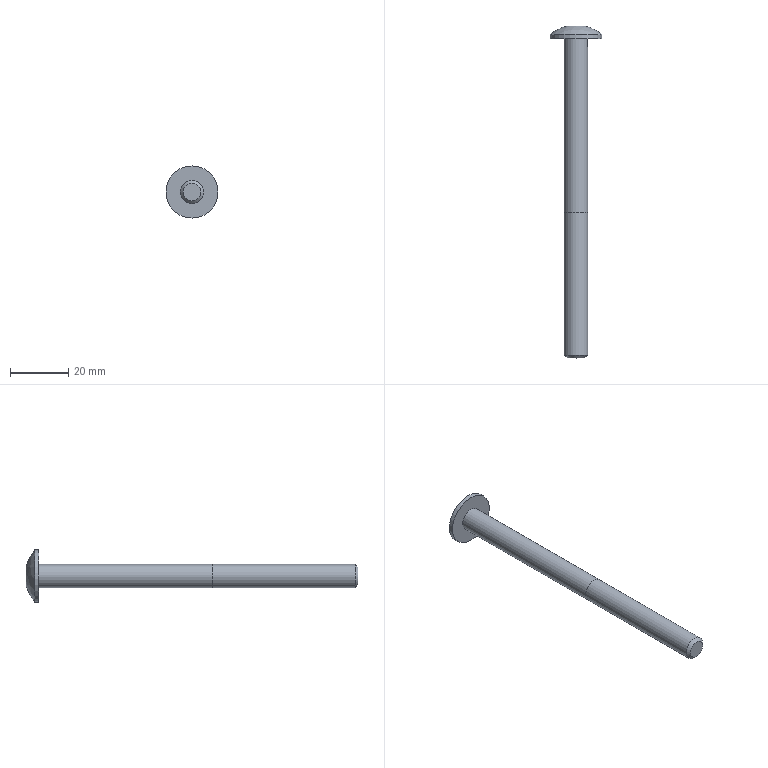Part | STEP file | PN_0020 | 1 solid | 14 faces | box 18 x 114.451 x 18 mm | volume 6223 mm3 | plane 9 | cylinder 3 | sphere 1 | cone 1 | commonest cylinder face diameters 8 x2 18 x1
STEP:
#1=CARTESIAN_POINT('',(0.,0.,0.));
#2=DIRECTION('',(0.,0.,1.));
#3=DIRECTION('',(1.,0.,0.));
#4=AXIS2_PLACEMENT_3D('',#1,#2,#3);
#5=CARTESIAN_POINT('',(0.,0.,4.));
#6=VERTEX_POINT('',#5);
#7=CARTESIAN_POINT('',(0.,0.,0.));
#8=DIRECTION('',(0.,-1.,0.));
#9=DIRECTION('',(0.,0.,1.));
#10=AXIS2_PLACEMENT_3D('',#7,#8,#9);
#11=CIRCLE('',#10,4.);
#12=CARTESIAN_POINT('',(0.,-110.,0.));
#13=DIRECTION('',(0.,1.,0.));
#14=DIRECTION('',(0.,0.,1.));
#15=AXIS2_PLACEMENT_3D('',#12,#13,#14);
#16=CYLINDRICAL_SURFACE('',#15,4.);
#17=CARTESIAN_POINT('',(6.283,110.));
#18=DIRECTION('',(-1.,0.));
#19=VECTOR('',#18,1.);
#20=LINE('',#17,#19);
#21=(GEOMETRIC_REPRESENTATION_CONTEXT(2)PARAMETRIC_REPRESENTATION_CONTEXT()REPRESENTATION_CONTEXT('',''));
#22=DEFINITIONAL_REPRESENTATION('',(#20),#21);
#23=PCURVE('',#16,#22);
#24=CARTESIAN_POINT('',(0.,0.,0.));
#25=DIRECTION('',(0.,1.,0.));
#26=DIRECTION('',(0.,0.,1.));
#27=AXIS2_PLACEMENT_3D('',#24,#25,#26);
#28=PLANE('',#27);
#29=CARTESIAN_POINT('',(4.,0.));
#30=CARTESIAN_POINT('',(4.,-6.928));
#31=CARTESIAN_POINT('',(-2.,-3.464));
#32=CARTESIAN_POINT('',(-8.,0.));
#33=CARTESIAN_POINT('',(-2.,3.464));
#34=CARTESIAN_POINT('',(4.,6.928));
#35=CARTESIAN_POINT('',(4.,0.));
#36=(BOUNDED_CURVE()B_SPLINE_CURVE(2,(#29,#30,#31,#32,#33,#34,#35),.UNSPECIFIED.,.T.,.F.)B_SPLINE_CURVE_WITH_KNOTS((1,2,2,2,2,1),(-2.094,0.,2.094,4.189,6.283,8.378),.UNSPECIFIED.)CURVE()GEOMETRIC_REPRESENTATION_ITEM()RATIONAL_B_SPLINE_CURVE((1.,0.5,1.,0.5,1.,0.5,1.))REPRESENTATION_ITEM(''));
#37=(GEOMETRIC_REPRESENTATION_CONTEXT(2)PARAMETRIC_REPRESENTATION_CONTEXT()REPRESENTATION_CONTEXT('',''));
#38=DEFINITIONAL_REPRESENTATION('',(#36),#37);
#39=PCURVE('',#28,#38);
#40=SURFACE_CURVE('',#11,(#23,#39),.PCURVE_S1.);
#41=EDGE_CURVE('',#6,#6,#40,.T.);
#42=ORIENTED_EDGE('',*,*,#41,.T.);
#43=CARTESIAN_POINT('',(0.,-60.,4.));
#44=VERTEX_POINT('',#43);
#45=CARTESIAN_POINT('',(0.,-60.,4.));
#46=CARTESIAN_POINT('',(0.,0.,4.));
#47=B_SPLINE_CURVE_WITH_KNOTS('',1,(#45,#46),.UNSPECIFIED.,.F.,.F.,(2,2),(50.,110.),.PIECEWISE_BEZIER_KNOTS.);
#48=CARTESIAN_POINT('',(0.,0.));
#49=DIRECTION('',(0.,1.));
#50=VECTOR('',#49,1.);
#51=LINE('',#48,#50);
#52=(GEOMETRIC_REPRESENTATION_CONTEXT(2)PARAMETRIC_REPRESENTATION_CONTEXT()REPRESENTATION_CONTEXT('',''));
#53=DEFINITIONAL_REPRESENTATION('',(#51),#52);
#54=PCURVE('',#16,#53);
#55=CARTESIAN_POINT('',(6.283,0.));
#56=DIRECTION('',(0.,1.));
#57=VECTOR('',#56,1.);
#58=LINE('',#55,#57);
#59=(GEOMETRIC_REPRESENTATION_CONTEXT(2)PARAMETRIC_REPRESENTATION_CONTEXT()REPRESENTATION_CONTEXT('',''));
#60=DEFINITIONAL_REPRESENTATION('',(#58),#59);
#61=PCURVE('',#16,#60);
#62=SEAM_CURVE('',#47,(#54,#61),.PCURVE_S1.);
#63=EDGE_CURVE('',#44,#6,#62,.T.);
#64=ORIENTED_EDGE('',*,*,#63,.F.);
#65=CARTESIAN_POINT('',(0.,-60.,-4.));
#66=VERTEX_POINT('',#65);
#67=CARTESIAN_POINT('',(0.,-60.,0.));
#68=DIRECTION('',(0.,-1.,0.));
#69=DIRECTION('',(0.,0.,-1.));
#70=AXIS2_PLACEMENT_3D('',#67,#68,#69);
#71=CIRCLE('',#70,4.);
#72=CARTESIAN_POINT('',(3.142,50.));
#73=DIRECTION('',(-1.,0.));
#74=VECTOR('',#73,1.);
#75=LINE('',#72,#74);
#76=(GEOMETRIC_REPRESENTATION_CONTEXT(2)PARAMETRIC_REPRESENTATION_CONTEXT()REPRESENTATION_CONTEXT('',''));
#77=DEFINITIONAL_REPRESENTATION('',(#75),#76);
#78=PCURVE('',#16,#77);
#79=CARTESIAN_POINT('',(0.,-110.,0.));
#80=DIRECTION('',(0.,1.,0.));
#81=DIRECTION('',(0.,0.,1.));
#82=AXIS2_PLACEMENT_3D('',#79,#80,#81);
#83=CYLINDRICAL_SURFACE('',#82,4.);
#84=CARTESIAN_POINT('',(9.425,50.));
#85=DIRECTION('',(-1.,0.));
#86=VECTOR('',#85,1.);
#87=LINE('',#84,#86);
#88=(GEOMETRIC_REPRESENTATION_CONTEXT(2)PARAMETRIC_REPRESENTATION_CONTEXT()REPRESENTATION_CONTEXT('',''));
#89=DEFINITIONAL_REPRESENTATION('',(#87),#88);
#90=PCURVE('',#83,#89);
#91=SURFACE_CURVE('',#71,(#78,#90),.PCURVE_S1.);
#92=EDGE_CURVE('',#66,#44,#91,.T.);
#93=ORIENTED_EDGE('',*,*,#92,.F.);
#94=CARTESIAN_POINT('',(0.,-60.,0.));
#95=DIRECTION('',(0.,-1.,0.));
#96=DIRECTION('',(0.,0.,-1.));
#97=AXIS2_PLACEMENT_3D('',#94,#95,#96);
#98=CIRCLE('',#97,4.);
#99=CARTESIAN_POINT('',(9.425,50.));
#100=DIRECTION('',(-1.,0.));
#101=VECTOR('',#100,1.);
#102=LINE('',#99,#101);
#103=(GEOMETRIC_REPRESENTATION_CONTEXT(2)PARAMETRIC_REPRESENTATION_CONTEXT()REPRESENTATION_CONTEXT('',''));
#104=DEFINITIONAL_REPRESENTATION('',(#102),#103);
#105=PCURVE('',#16,#104);
#106=CARTESIAN_POINT('',(9.425,50.));
#107=DIRECTION('',(-1.,0.));
#108=VECTOR('',#107,1.);
#109=LINE('',#106,#108);
#110=(GEOMETRIC_REPRESENTATION_CONTEXT(2)PARAMETRIC_REPRESENTATION_CONTEXT()REPRESENTATION_CONTEXT('',''));
#111=DEFINITIONAL_REPRESENTATION('',(#109),#110);
#112=PCURVE('',#83,#111);
#113=SURFACE_CURVE('',#98,(#105,#112),.PCURVE_S1.);
#114=EDGE_CURVE('',#44,#66,#113,.T.);
#115=ORIENTED_EDGE('',*,*,#114,.F.);
#116=ORIENTED_EDGE('',*,*,#63,.T.);
#117=EDGE_LOOP('',(#42,#64,#93,#115,#116));
#118=FACE_BOUND('',#117,.T.);
#119=ADVANCED_FACE('',(#118),#16,.T.);
#120=CARTESIAN_POINT('',(0.,0.,9.));
#121=VERTEX_POINT('',#120);
#122=CARTESIAN_POINT('',(0.,0.,0.));
#123=DIRECTION('',(0.,1.,0.));
#124=DIRECTION('',(0.,0.,1.));
#125=AXIS2_PLACEMENT_3D('',#122,#123,#124);
#126=CIRCLE('',#125,9.);
#127=CARTESIAN_POINT('',(0.,0.));
#128=DIRECTION('',(1.,0.));
#129=AXIS2_PLACEMENT_2D('',#127,#128);
#130=CIRCLE('',#129,9.);
#131=(GEOMETRIC_REPRESENTATION_CONTEXT(2)PARAMETRIC_REPRESENTATION_CONTEXT()REPRESENTATION_CONTEXT('',''));
#132=DEFINITIONAL_REPRESENTATION('',(#130),#131);
#133=PCURVE('',#28,#132);
#134=CARTESIAN_POINT('',(0.,70.,0.));
#135=DIRECTION('',(0.,1.,0.));
#136=DIRECTION('',(0.,0.,1.));
#137=AXIS2_PLACEMENT_3D('',#134,#135,#136);
#138=CYLINDRICAL_SURFACE('',#137,9.);
#139=CARTESIAN_POINT('',(0.,-70.));
#140=DIRECTION('',(1.,0.));
#141=VECTOR('',#140,1.);
#142=LINE('',#139,#141);
#143=(GEOMETRIC_REPRESENTATION_CONTEXT(2)PARAMETRIC_REPRESENTATION_CONTEXT()REPRESENTATION_CONTEXT('',''));
#144=DEFINITIONAL_REPRESENTATION('',(#142),#143);
#145=PCURVE('',#138,#144);
#146=SURFACE_CURVE('',#126,(#133,#145),.PCURVE_S1.);
#147=EDGE_CURVE('',#121,#121,#146,.T.);
#148=ORIENTED_EDGE('',*,*,#147,.F.);
#149=EDGE_LOOP('',(#148));
#150=FACE_BOUND('',#149,.T.);
#151=ORIENTED_EDGE('',*,*,#41,.F.);
#152=EDGE_LOOP('',(#151));
#153=FACE_BOUND('',#152,.T.);
#154=ADVANCED_FACE('',(#150,#153),#28,.F.);
#155=CARTESIAN_POINT('',(0.,1.5,9.));
#156=VERTEX_POINT('',#155);
#157=CARTESIAN_POINT('',(0.,1.5,0.));
#158=DIRECTION('',(0.,1.,0.));
#159=DIRECTION('',(0.,0.,1.));
#160=AXIS2_PLACEMENT_3D('',#157,#158,#159);
#161=CIRCLE('',#160,9.);
#162=CARTESIAN_POINT('',(0.,-9.224,0.));
#163=DIRECTION('',(0.,0.,-1.));
#164=DIRECTION('',(1.,0.,0.));
#165=AXIS2_PLACEMENT_3D('',#162,#163,#164);
#166=SPHERICAL_SURFACE('',#165,14.);
#167=CARTESIAN_POINT('',(4.712,-0.6982));
#168=CARTESIAN_POINT('',(4.794,-0.6988));
#169=CARTESIAN_POINT('',(4.951,-0.6746));
#170=CARTESIAN_POINT('',(5.148,-0.5787));
#171=CARTESIAN_POINT('',(5.286,-0.4389));
#172=CARTESIAN_POINT('',(5.372,-0.2727));
#173=CARTESIAN_POINT('',(5.412,-0.09234));
#174=CARTESIAN_POINT('',(5.412,0.09234));
#175=CARTESIAN_POINT('',(5.372,0.2727));
#176=CARTESIAN_POINT('',(5.286,0.439));
#177=CARTESIAN_POINT('',(5.148,0.5786));
#178=CARTESIAN_POINT('',(4.952,0.6749));
#179=CARTESIAN_POINT('',(4.712,0.7099));
#180=CARTESIAN_POINT('',(4.473,0.6749));
#181=CARTESIAN_POINT('',(4.277,0.5786));
#182=CARTESIAN_POINT('',(4.138,0.439));
#183=CARTESIAN_POINT('',(4.053,0.2727));
#184=CARTESIAN_POINT('',(4.012,0.09234));
#185=CARTESIAN_POINT('',(4.012,-0.09234));
#186=CARTESIAN_POINT('',(4.053,-0.2727));
#187=CARTESIAN_POINT('',(4.138,-0.4389));
#188=CARTESIAN_POINT('',(4.277,-0.5787));
#189=CARTESIAN_POINT('',(4.474,-0.6746));
#190=CARTESIAN_POINT('',(4.63,-0.6988));
#191=CARTESIAN_POINT('',(4.712,-0.6982));
#192=B_SPLINE_CURVE_WITH_KNOTS('',3,(#167,#168,#169,#170,#171,#172,#173,#174,#175,#176,#177,#178,#179,#180,#181,#182,#183,#184,#185,#186,#187,#188,#189,#190,#191),.UNSPECIFIED.,.T.,.F.,(4,1,1,1,1,1,1,1,1,1,1,1,1,1,1,1,1,1,1,1,1,1,4),(0.,0.2856,0.5712,0.8568,1.142,1.428,1.714,1.999,2.285,2.57,2.856,3.142,3.427,3.713,3.998,4.284,4.57,4.855,5.141,5.426,5.712,5.998,6.283),.QUASI_UNIFORM_KNOTS.);
#193=(GEOMETRIC_REPRESENTATION_CONTEXT(2)PARAMETRIC_REPRESENTATION_CONTEXT()REPRESENTATION_CONTEXT('',''));
#194=DEFINITIONAL_REPRESENTATION('',(#192),#193);
#195=PCURVE('',#166,#194);
#196=CARTESIAN_POINT('',(0.,-68.5));
#197=DIRECTION('',(1.,0.));
#198=VECTOR('',#197,1.);
#199=LINE('',#196,#198);
#200=(GEOMETRIC_REPRESENTATION_CONTEXT(2)PARAMETRIC_REPRESENTATION_CONTEXT()REPRESENTATION_CONTEXT('',''));
#201=DEFINITIONAL_REPRESENTATION('',(#199),#200);
#202=PCURVE('',#138,#201);
#203=SURFACE_CURVE('',#161,(#195,#202),.PCURVE_S1.);
#204=EDGE_CURVE('',#156,#156,#203,.T.);
#205=ORIENTED_EDGE('',*,*,#204,.T.);
#206=EDGE_LOOP('',(#205));
#207=FACE_BOUND('',#206,.T.);
#208=CARTESIAN_POINT('',(0.,4.341,-3.464));
#209=VERTEX_POINT('',#208);
#210=CARTESIAN_POINT('',(-3.,4.341,-1.732));
#211=VERTEX_POINT('',#210);
#212=CARTESIAN_POINT('',(-1.5,-9.224,-2.598));
#213=DIRECTION('',(0.5,0.,0.866));
#214=DIRECTION('',(0.866,0.,-0.5));
#215=AXIS2_PLACEMENT_3D('',#212,#213,#214);
#216=CIRCLE('',#215,13.675);
#217=CARTESIAN_POINT('',(4.712,0.25));
#218=CARTESIAN_POINT('',(4.709,0.2481));
#219=CARTESIAN_POINT('',(4.702,0.2443));
#220=CARTESIAN_POINT('',(4.692,0.2385));
#221=CARTESIAN_POINT('',(4.682,0.2327));
#222=CARTESIAN_POINT('',(4.673,0.2269));
#223=CARTESIAN_POINT('',(4.663,0.2212));
#224=CARTESIAN_POINT('',(4.653,0.2154));
#225=CARTESIAN_POINT('',(4.643,0.2097));
#226=CARTESIAN_POINT('',(4.633,0.2039));
#227=CARTESIAN_POINT('',(4.623,0.1981));
#228=CARTESIAN_POINT('',(4.613,0.1924));
#229=CARTESIAN_POINT('',(4.603,0.1867));
#230=CARTESIAN_POINT('',(4.593,0.1809));
#231=CARTESIAN_POINT('',(4.583,0.1752));
#232=CARTESIAN_POINT('',(4.574,0.1695));
#233=CARTESIAN_POINT('',(4.564,0.1638));
#234=CARTESIAN_POINT('',(4.554,0.1581));
#235=CARTESIAN_POINT('',(4.544,0.1524));
#236=CARTESIAN_POINT('',(4.534,0.1467));
#237=CARTESIAN_POINT('',(4.524,0.141));
#238=CARTESIAN_POINT('',(4.514,0.1353));
#239=CARTESIAN_POINT('',(4.505,0.1297));
#240=CARTESIAN_POINT('',(4.498,0.1259));
#241=CARTESIAN_POINT('',(4.495,0.124));
#242=B_SPLINE_CURVE_WITH_KNOTS('',3,(#217,#218,#219,#220,#221,#222,#223,#224,#225,#226,#227,#228,#229,#230,#231,#232,#233,#234,#235,#236,#237,#238,#239,#240,#241),.UNSPECIFIED.,.F.,.F.,(4,1,1,1,1,1,1,1,1,1,1,1,1,1,1,1,1,1,1,1,1,1,4),(1.444,1.455,1.467,1.478,1.49,1.502,1.513,1.525,1.536,1.548,1.559,1.571,1.582,1.594,1.605,1.617,1.629,1.64,1.652,1.663,1.675,1.686,1.698),.QUASI_UNIFORM_KNOTS.);
#243=(GEOMETRIC_REPRESENTATION_CONTEXT(2)PARAMETRIC_REPRESENTATION_CONTEXT()REPRESENTATION_CONTEXT('',''));
#244=DEFINITIONAL_REPRESENTATION('',(#242),#243);
#245=PCURVE('',#166,#244);
#246=CARTESIAN_POINT('',(-3.,1.,-1.732));
#247=DIRECTION('',(0.5,0.,0.866));
#248=DIRECTION('',(0.866,0.,-0.5));
#249=AXIS2_PLACEMENT_3D('',#246,#247,#248);
#250=PLANE('',#249);
#251=CARTESIAN_POINT('',(1.732,-10.224));
#252=DIRECTION('',(1.,0.));
#253=AXIS2_PLACEMENT_2D('',#251,#252);
#254=CIRCLE('',#253,13.675);
#255=(GEOMETRIC_REPRESENTATION_CONTEXT(2)PARAMETRIC_REPRESENTATION_CONTEXT()REPRESENTATION_CONTEXT('',''));
#256=DEFINITIONAL_REPRESENTATION('',(#254),#255);
#257=PCURVE('',#250,#256);
#258=SURFACE_CURVE('',#216,(#245,#257),.PCURVE_S1.);
#259=EDGE_CURVE('',#209,#211,#258,.T.);
#260=ORIENTED_EDGE('',*,*,#259,.F.);
#261=CARTESIAN_POINT('',(3.,4.341,-1.732));
#262=VERTEX_POINT('',#261);
#263=CARTESIAN_POINT('',(1.5,-9.224,-2.598));
#264=DIRECTION('',(-0.5,0.,0.866));
#265=DIRECTION('',(0.866,0.,0.5));
#266=AXIS2_PLACEMENT_3D('',#263,#264,#265);
#267=CIRCLE('',#266,13.675);
#268=CARTESIAN_POINT('',(4.93,0.124));
#269=CARTESIAN_POINT('',(4.927,0.1259));
#270=CARTESIAN_POINT('',(4.92,0.1297));
#271=CARTESIAN_POINT('',(4.91,0.1353));
#272=CARTESIAN_POINT('',(4.901,0.141));
#273=CARTESIAN_POINT('',(4.891,0.1467));
#274=CARTESIAN_POINT('',(4.881,0.1524));
#275=CARTESIAN_POINT('',(4.871,0.1581));
#276=CARTESIAN_POINT('',(4.861,0.1638));
#277=CARTESIAN_POINT('',(4.851,0.1695));
#278=CARTESIAN_POINT('',(4.841,0.1752));
#279=CARTESIAN_POINT('',(4.832,0.1809));
#280=CARTESIAN_POINT('',(4.822,0.1867));
#281=CARTESIAN_POINT('',(4.812,0.1924));
#282=CARTESIAN_POINT('',(4.802,0.1981));
#283=CARTESIAN_POINT('',(4.792,0.2039));
#284=CARTESIAN_POINT('',(4.782,0.2097));
#285=CARTESIAN_POINT('',(4.772,0.2154));
#286=CARTESIAN_POINT('',(4.762,0.2212));
#287=CARTESIAN_POINT('',(4.752,0.2269));
#288=CARTESIAN_POINT('',(4.742,0.2327));
#289=CARTESIAN_POINT('',(4.732,0.2385));
#290=CARTESIAN_POINT('',(4.722,0.2443));
#291=CARTESIAN_POINT('',(4.716,0.2481));
#292=CARTESIAN_POINT('',(4.712,0.25));
#293=B_SPLINE_CURVE_WITH_KNOTS('',3,(#268,#269,#270,#271,#272,#273,#274,#275,#276,#277,#278,#279,#280,#281,#282,#283,#284,#285,#286,#287,#288,#289,#290,#291,#292),.UNSPECIFIED.,.F.,.F.,(4,1,1,1,1,1,1,1,1,1,1,1,1,1,1,1,1,1,1,1,1,1,4),(1.444,1.455,1.467,1.478,1.49,1.502,1.513,1.525,1.536,1.548,1.559,1.571,1.582,1.594,1.605,1.617,1.629,1.64,1.652,1.663,1.675,1.686,1.698),.QUASI_UNIFORM_KNOTS.);
#294=(GEOMETRIC_REPRESENTATION_CONTEXT(2)PARAMETRIC_REPRESENTATION_CONTEXT()REPRESENTATION_CONTEXT('',''));
#295=DEFINITIONAL_REPRESENTATION('',(#293),#294);
#296=PCURVE('',#166,#295);
#297=CARTESIAN_POINT('',(0.,1.,-3.464));
#298=DIRECTION('',(-0.5,0.,0.866));
#299=DIRECTION('',(0.866,0.,0.5));
#300=AXIS2_PLACEMENT_3D('',#297,#298,#299);
#301=PLANE('',#300);
#302=CARTESIAN_POINT('',(1.732,-10.224));
#303=DIRECTION('',(1.,0.));
#304=AXIS2_PLACEMENT_2D('',#302,#303);
#305=CIRCLE('',#304,13.675);
#306=(GEOMETRIC_REPRESENTATION_CONTEXT(2)PARAMETRIC_REPRESENTATION_CONTEXT()REPRESENTATION_CONTEXT('',''));
#307=DEFINITIONAL_REPRESENTATION('',(#305),#306);
#308=PCURVE('',#301,#307);
#309=SURFACE_CURVE('',#267,(#296,#308),.PCURVE_S1.);
#310=EDGE_CURVE('',#262,#209,#309,.T.);
#311=ORIENTED_EDGE('',*,*,#310,.F.);
#312=CARTESIAN_POINT('',(3.,4.341,1.732));
#313=VERTEX_POINT('',#312);
#314=CARTESIAN_POINT('',(3.,-9.224,0.));
#315=DIRECTION('',(-1.,0.,0.));
#316=DIRECTION('',(0.,0.,1.));
#317=AXIS2_PLACEMENT_3D('',#314,#315,#316);
#318=CIRCLE('',#317,13.675);
#319=CARTESIAN_POINT('',(4.93,-0.124));
#320=CARTESIAN_POINT('',(4.93,-0.1203));
#321=CARTESIAN_POINT('',(4.93,-0.1128));
#322=CARTESIAN_POINT('',(4.929,-0.1015));
#323=CARTESIAN_POINT('',(4.929,-0.09021));
#324=CARTESIAN_POINT('',(4.929,-0.07894));
#325=CARTESIAN_POINT('',(4.929,-0.06766));
#326=CARTESIAN_POINT('',(4.929,-0.05639));
#327=CARTESIAN_POINT('',(4.929,-0.04511));
#328=CARTESIAN_POINT('',(4.928,-0.03383));
#329=CARTESIAN_POINT('',(4.928,-0.02255));
#330=CARTESIAN_POINT('',(4.928,-0.01128));
#331=CARTESIAN_POINT('',(4.928,0.));
#332=CARTESIAN_POINT('',(4.928,0.01128));
#333=CARTESIAN_POINT('',(4.928,0.02255));
#334=CARTESIAN_POINT('',(4.928,0.03383));
#335=CARTESIAN_POINT('',(4.929,0.04511));
#336=CARTESIAN_POINT('',(4.929,0.05639));
#337=CARTESIAN_POINT('',(4.929,0.06766));
#338=CARTESIAN_POINT('',(4.929,0.07894));
#339=CARTESIAN_POINT('',(4.929,0.09021));
#340=CARTESIAN_POINT('',(4.929,0.1015));
#341=CARTESIAN_POINT('',(4.93,0.1128));
#342=CARTESIAN_POINT('',(4.93,0.1203));
#343=CARTESIAN_POINT('',(4.93,0.124));
#344=B_SPLINE_CURVE_WITH_KNOTS('',3,(#319,#320,#321,#322,#323,#324,#325,#326,#327,#328,#329,#330,#331,#332,#333,#334,#335,#336,#337,#338,#339,#340,#341,#342,#343),.UNSPECIFIED.,.F.,.F.,(4,1,1,1,1,1,1,1,1,1,1,1,1,1,1,1,1,1,1,1,1,1,4),(1.444,1.455,1.467,1.478,1.49,1.502,1.513,1.525,1.536,1.548,1.559,1.571,1.582,1.594,1.605,1.617,1.629,1.64,1.652,1.663,1.675,1.686,1.698),.QUASI_UNIFORM_KNOTS.);
#345=(GEOMETRIC_REPRESENTATION_CONTEXT(2)PARAMETRIC_REPRESENTATION_CONTEXT()REPRESENTATION_CONTEXT('',''));
#346=DEFINITIONAL_REPRESENTATION('',(#344),#345);
#347=PCURVE('',#166,#346);
#348=CARTESIAN_POINT('',(3.,1.,-1.732));
#349=DIRECTION('',(-1.,0.,0.));
#350=DIRECTION('',(0.,0.,1.));
#351=AXIS2_PLACEMENT_3D('',#348,#349,#350);
#352=PLANE('',#351);
#353=CARTESIAN_POINT('',(1.732,-10.224));
#354=DIRECTION('',(1.,0.));
#355=AXIS2_PLACEMENT_2D('',#353,#354);
#356=CIRCLE('',#355,13.675);
#357=(GEOMETRIC_REPRESENTATION_CONTEXT(2)PARAMETRIC_REPRESENTATION_CONTEXT()REPRESENTATION_CONTEXT('',''));
#358=DEFINITIONAL_REPRESENTATION('',(#356),#357);
#359=PCURVE('',#352,#358);
#360=SURFACE_CURVE('',#318,(#347,#359),.PCURVE_S1.);
#361=EDGE_CURVE('',#313,#262,#360,.T.);
#362=ORIENTED_EDGE('',*,*,#361,.F.);
#363=CARTESIAN_POINT('',(0.,4.341,3.464));
#364=VERTEX_POINT('',#363);
#365=CARTESIAN_POINT('',(1.5,-9.224,2.598));
#366=DIRECTION('',(-0.5,0.,-0.866));
#367=DIRECTION('',(-0.866,0.,0.5));
#368=AXIS2_PLACEMENT_3D('',#365,#366,#367);
#369=CIRCLE('',#368,13.675);
#370=CARTESIAN_POINT('',(4.712,-0.25));
#371=CARTESIAN_POINT('',(4.716,-0.2481));
#372=CARTESIAN_POINT('',(4.722,-0.2443));
#373=CARTESIAN_POINT('',(4.732,-0.2385));
#374=CARTESIAN_POINT('',(4.742,-0.2327));
#375=CARTESIAN_POINT('',(4.752,-0.2269));
#376=CARTESIAN_POINT('',(4.762,-0.2212));
#377=CARTESIAN_POINT('',(4.772,-0.2154));
#378=CARTESIAN_POINT('',(4.782,-0.2097));
#379=CARTESIAN_POINT('',(4.792,-0.2039));
#380=CARTESIAN_POINT('',(4.802,-0.1981));
#381=CARTESIAN_POINT('',(4.812,-0.1924));
#382=CARTESIAN_POINT('',(4.822,-0.1867));
#383=CARTESIAN_POINT('',(4.832,-0.1809));
#384=CARTESIAN_POINT('',(4.841,-0.1752));
#385=CARTESIAN_POINT('',(4.851,-0.1695));
#386=CARTESIAN_POINT('',(4.861,-0.1638));
#387=CARTESIAN_POINT('',(4.871,-0.1581));
#388=CARTESIAN_POINT('',(4.881,-0.1524));
#389=CARTESIAN_POINT('',(4.891,-0.1467));
#390=CARTESIAN_POINT('',(4.901,-0.141));
#391=CARTESIAN_POINT('',(4.91,-0.1353));
#392=CARTESIAN_POINT('',(4.92,-0.1297));
#393=CARTESIAN_POINT('',(4.927,-0.1259));
#394=CARTESIAN_POINT('',(4.93,-0.124));
#395=B_SPLINE_CURVE_WITH_KNOTS('',3,(#370,#371,#372,#373,#374,#375,#376,#377,#378,#379,#380,#381,#382,#383,#384,#385,#386,#387,#388,#389,#390,#391,#392,#393,#394),.UNSPECIFIED.,.F.,.F.,(4,1,1,1,1,1,1,1,1,1,1,1,1,1,1,1,1,1,1,1,1,1,4),(1.444,1.455,1.467,1.478,1.49,1.502,1.513,1.525,1.536,1.548,1.559,1.571,1.582,1.594,1.605,1.617,1.629,1.64,1.652,1.663,1.675,1.686,1.698),.QUASI_UNIFORM_KNOTS.);
#396=(GEOMETRIC_REPRESENTATION_CONTEXT(2)PARAMETRIC_REPRESENTATION_CONTEXT()REPRESENTATION_CONTEXT('',''));
#397=DEFINITIONAL_REPRESENTATION('',(#395),#396);
#398=PCURVE('',#166,#397);
#399=CARTESIAN_POINT('',(3.,1.,1.732));
#400=DIRECTION('',(-0.5,0.,-0.866));
#401=DIRECTION('',(-0.866,0.,0.5));
#402=AXIS2_PLACEMENT_3D('',#399,#400,#401);
#403=PLANE('',#402);
#404=CARTESIAN_POINT('',(1.732,-10.224));
#405=DIRECTION('',(1.,0.));
#406=AXIS2_PLACEMENT_2D('',#404,#405);
#407=CIRCLE('',#406,13.675);
#408=(GEOMETRIC_REPRESENTATION_CONTEXT(2)PARAMETRIC_REPRESENTATION_CONTEXT()REPRESENTATION_CONTEXT('',''));
#409=DEFINITIONAL_REPRESENTATION('',(#407),#408);
#410=PCURVE('',#403,#409);
#411=SURFACE_CURVE('',#369,(#398,#410),.PCURVE_S1.);
#412=EDGE_CURVE('',#364,#313,#411,.T.);
#413=ORIENTED_EDGE('',*,*,#412,.F.);
#414=CARTESIAN_POINT('',(-3.,4.341,1.732));
#415=VERTEX_POINT('',#414);
#416=CARTESIAN_POINT('',(-1.5,-9.224,2.598));
#417=DIRECTION('',(0.5,0.,-0.866));
#418=DIRECTION('',(-0.866,0.,-0.5));
#419=AXIS2_PLACEMENT_3D('',#416,#417,#418);
#420=CIRCLE('',#419,13.675);
#421=CARTESIAN_POINT('',(4.495,-0.124));
#422=CARTESIAN_POINT('',(4.498,-0.1259));
#423=CARTESIAN_POINT('',(4.505,-0.1297));
#424=CARTESIAN_POINT('',(4.514,-0.1353));
#425=CARTESIAN_POINT('',(4.524,-0.141));
#426=CARTESIAN_POINT('',(4.534,-0.1467));
#427=CARTESIAN_POINT('',(4.544,-0.1524));
#428=CARTESIAN_POINT('',(4.554,-0.1581));
#429=CARTESIAN_POINT('',(4.564,-0.1638));
#430=CARTESIAN_POINT('',(4.574,-0.1695));
#431=CARTESIAN_POINT('',(4.583,-0.1752));
#432=CARTESIAN_POINT('',(4.593,-0.1809));
#433=CARTESIAN_POINT('',(4.603,-0.1867));
#434=CARTESIAN_POINT('',(4.613,-0.1924));
#435=CARTESIAN_POINT('',(4.623,-0.1981));
#436=CARTESIAN_POINT('',(4.633,-0.2039));
#437=CARTESIAN_POINT('',(4.643,-0.2097));
#438=CARTESIAN_POINT('',(4.653,-0.2154));
#439=CARTESIAN_POINT('',(4.663,-0.2212));
#440=CARTESIAN_POINT('',(4.673,-0.2269));
#441=CARTESIAN_POINT('',(4.682,-0.2327));
#442=CARTESIAN_POINT('',(4.692,-0.2385));
#443=CARTESIAN_POINT('',(4.702,-0.2443));
#444=CARTESIAN_POINT('',(4.709,-0.2481));
#445=CARTESIAN_POINT('',(4.712,-0.25));
#446=B_SPLINE_CURVE_WITH_KNOTS('',3,(#421,#422,#423,#424,#425,#426,#427,#428,#429,#430,#431,#432,#433,#434,#435,#436,#437,#438,#439,#440,#441,#442,#443,#444,#445),.UNSPECIFIED.,.F.,.F.,(4,1,1,1,1,1,1,1,1,1,1,1,1,1,1,1,1,1,1,1,1,1,4),(1.444,1.455,1.467,1.478,1.49,1.502,1.513,1.525,1.536,1.548,1.559,1.571,1.582,1.594,1.605,1.617,1.629,1.64,1.652,1.663,1.675,1.686,1.698),.QUASI_UNIFORM_KNOTS.);
#447=(GEOMETRIC_REPRESENTATION_CONTEXT(2)PARAMETRIC_REPRESENTATION_CONTEXT()REPRESENTATION_CONTEXT('',''));
#448=DEFINITIONAL_REPRESENTATION('',(#446),#447);
#449=PCURVE('',#166,#448);
#450=CARTESIAN_POINT('',(0.,1.,3.464));
#451=DIRECTION('',(0.5,0.,-0.866));
#452=DIRECTION('',(-0.866,0.,-0.5));
#453=AXIS2_PLACEMENT_3D('',#450,#451,#452);
#454=PLANE('',#453);
#455=CARTESIAN_POINT('',(1.732,-10.224));
#456=DIRECTION('',(1.,0.));
#457=AXIS2_PLACEMENT_2D('',#455,#456);
#458=CIRCLE('',#457,13.675);
#459=(GEOMETRIC_REPRESENTATION_CONTEXT(2)PARAMETRIC_REPRESENTATION_CONTEXT()REPRESENTATION_CONTEXT('',''));
#460=DEFINITIONAL_REPRESENTATION('',(#458),#459);
#461=PCURVE('',#454,#460);
#462=SURFACE_CURVE('',#420,(#449,#461),.PCURVE_S1.);
#463=EDGE_CURVE('',#415,#364,#462,.T.);
#464=ORIENTED_EDGE('',*,*,#463,.F.);
#465=CARTESIAN_POINT('',(-3.,-9.224,0.));
#466=DIRECTION('',(1.,0.,0.));
#467=DIRECTION('',(0.,0.,-1.));
#468=AXIS2_PLACEMENT_3D('',#465,#466,#467);
#469=CIRCLE('',#468,13.675);
#470=CARTESIAN_POINT('',(4.495,0.124));
#471=CARTESIAN_POINT('',(4.495,0.1203));
#472=CARTESIAN_POINT('',(4.495,0.1128));
#473=CARTESIAN_POINT('',(4.495,0.1015));
#474=CARTESIAN_POINT('',(4.496,0.09021));
#475=CARTESIAN_POINT('',(4.496,0.07894));
#476=CARTESIAN_POINT('',(4.496,0.06766));
#477=CARTESIAN_POINT('',(4.496,0.05639));
#478=CARTESIAN_POINT('',(4.496,0.04511));
#479=CARTESIAN_POINT('',(4.496,0.03383));
#480=CARTESIAN_POINT('',(4.496,0.02255));
#481=CARTESIAN_POINT('',(4.496,0.01128));
#482=CARTESIAN_POINT('',(4.496,0.));
#483=CARTESIAN_POINT('',(4.496,-0.01128));
#484=CARTESIAN_POINT('',(4.496,-0.02255));
#485=CARTESIAN_POINT('',(4.496,-0.03383));
#486=CARTESIAN_POINT('',(4.496,-0.04511));
#487=CARTESIAN_POINT('',(4.496,-0.05639));
#488=CARTESIAN_POINT('',(4.496,-0.06766));
#489=CARTESIAN_POINT('',(4.496,-0.07894));
#490=CARTESIAN_POINT('',(4.496,-0.09021));
#491=CARTESIAN_POINT('',(4.495,-0.1015));
#492=CARTESIAN_POINT('',(4.495,-0.1128));
#493=CARTESIAN_POINT('',(4.495,-0.1203));
#494=CARTESIAN_POINT('',(4.495,-0.124));
#495=B_SPLINE_CURVE_WITH_KNOTS('',3,(#470,#471,#472,#473,#474,#475,#476,#477,#478,#479,#480,#481,#482,#483,#484,#485,#486,#487,#488,#489,#490,#491,#492,#493,#494),.UNSPECIFIED.,.F.,.F.,(4,1,1,1,1,1,1,1,1,1,1,1,1,1,1,1,1,1,1,1,1,1,4),(1.444,1.455,1.467,1.478,1.49,1.502,1.513,1.525,1.536,1.548,1.559,1.571,1.582,1.594,1.605,1.617,1.629,1.64,1.652,1.663,1.675,1.686,1.698),.QUASI_UNIFORM_KNOTS.);
#496=(GEOMETRIC_REPRESENTATION_CONTEXT(2)PARAMETRIC_REPRESENTATION_CONTEXT()REPRESENTATION_CONTEXT('',''));
#497=DEFINITIONAL_REPRESENTATION('',(#495),#496);
#498=PCURVE('',#166,#497);
#499=CARTESIAN_POINT('',(-3.,1.,1.732));
#500=DIRECTION('',(1.,0.,0.));
#501=DIRECTION('',(0.,0.,-1.));
#502=AXIS2_PLACEMENT_3D('',#499,#500,#501);
#503=PLANE('',#502);
#504=CARTESIAN_POINT('',(1.732,-10.224));
#505=DIRECTION('',(1.,0.));
#506=AXIS2_PLACEMENT_2D('',#504,#505);
#507=CIRCLE('',#506,13.675);
#508=(GEOMETRIC_REPRESENTATION_CONTEXT(2)PARAMETRIC_REPRESENTATION_CONTEXT()REPRESENTATION_CONTEXT('',''));
#509=DEFINITIONAL_REPRESENTATION('',(#507),#508);
#510=PCURVE('',#503,#509);
#511=SURFACE_CURVE('',#469,(#498,#510),.PCURVE_S1.);
#512=EDGE_CURVE('',#211,#415,#511,.T.);
#513=ORIENTED_EDGE('',*,*,#512,.F.);
#514=EDGE_LOOP('',(#260,#311,#362,#413,#464,#513));
#515=FACE_BOUND('',#514,.T.);
#516=ADVANCED_FACE('',(#207,#515),#166,.T.);
#517=ORIENTED_EDGE('',*,*,#204,.F.);
#518=CARTESIAN_POINT('',(0.,0.,9.));
#519=CARTESIAN_POINT('',(0.,1.5,9.));
#520=B_SPLINE_CURVE_WITH_KNOTS('',1,(#518,#519),.UNSPECIFIED.,.F.,.F.,(2,2),(-70.,-68.5),.PIECEWISE_BEZIER_KNOTS.);
#521=CARTESIAN_POINT('',(0.,0.));
#522=DIRECTION('',(0.,1.));
#523=VECTOR('',#522,1.);
#524=LINE('',#521,#523);
#525=(GEOMETRIC_REPRESENTATION_CONTEXT(2)PARAMETRIC_REPRESENTATION_CONTEXT()REPRESENTATION_CONTEXT('',''));
#526=DEFINITIONAL_REPRESENTATION('',(#524),#525);
#527=PCURVE('',#138,#526);
#528=CARTESIAN_POINT('',(6.283,0.));
#529=DIRECTION('',(0.,1.));
#530=VECTOR('',#529,1.);
#531=LINE('',#528,#530);
#532=(GEOMETRIC_REPRESENTATION_CONTEXT(2)PARAMETRIC_REPRESENTATION_CONTEXT()REPRESENTATION_CONTEXT('',''));
#533=DEFINITIONAL_REPRESENTATION('',(#531),#532);
#534=PCURVE('',#138,#533);
#535=SEAM_CURVE('',#520,(#527,#534),.PCURVE_S1.);
#536=EDGE_CURVE('',#121,#156,#535,.T.);
#537=ORIENTED_EDGE('',*,*,#536,.F.);
#538=ORIENTED_EDGE('',*,*,#147,.T.);
#539=ORIENTED_EDGE('',*,*,#536,.T.);
#540=EDGE_LOOP('',(#517,#537,#538,#539));
#541=FACE_BOUND('',#540,.T.);
#542=ADVANCED_FACE('',(#541),#138,.T.);
#543=ORIENTED_EDGE('',*,*,#259,.T.);
#544=CARTESIAN_POINT('',(-3.,1.,-1.732));
#545=VERTEX_POINT('',#544);
#546=CARTESIAN_POINT('',(-3.,1.,-1.732));
#547=DIRECTION('',(0.,1.,0.));
#548=VECTOR('',#547,1.);
#549=LINE('',#546,#548);
#550=CARTESIAN_POINT('',(0.,0.));
#551=DIRECTION('',(0.,1.));
#552=VECTOR('',#551,1.);
#553=LINE('',#550,#552);
#554=(GEOMETRIC_REPRESENTATION_CONTEXT(2)PARAMETRIC_REPRESENTATION_CONTEXT()REPRESENTATION_CONTEXT('',''));
#555=DEFINITIONAL_REPRESENTATION('',(#553),#554);
#556=PCURVE('',#250,#555);
#557=CARTESIAN_POINT('',(3.464,0.));
#558=DIRECTION('',(0.,1.));
#559=VECTOR('',#558,1.);
#560=LINE('',#557,#559);
#561=(GEOMETRIC_REPRESENTATION_CONTEXT(2)PARAMETRIC_REPRESENTATION_CONTEXT()REPRESENTATION_CONTEXT('',''));
#562=DEFINITIONAL_REPRESENTATION('',(#560),#561);
#563=PCURVE('',#503,#562);
#564=SURFACE_CURVE('',#549,(#556,#563),.PCURVE_S1.);
#565=EDGE_CURVE('',#545,#211,#564,.T.);
#566=ORIENTED_EDGE('',*,*,#565,.F.);
#567=CARTESIAN_POINT('',(0.,1.,-3.464));
#568=VERTEX_POINT('',#567);
#569=CARTESIAN_POINT('',(-3.,1.,-1.732));
#570=DIRECTION('',(0.866,0.,-0.5));
#571=VECTOR('',#570,1.);
#572=LINE('',#569,#571);
#573=CARTESIAN_POINT('',(0.,0.));
#574=DIRECTION('',(1.,0.));
#575=VECTOR('',#574,1.);
#576=LINE('',#573,#575);
#577=(GEOMETRIC_REPRESENTATION_CONTEXT(2)PARAMETRIC_REPRESENTATION_CONTEXT()REPRESENTATION_CONTEXT('',''));
#578=DEFINITIONAL_REPRESENTATION('',(#576),#577);
#579=PCURVE('',#250,#578);
#580=CARTESIAN_POINT('',(-3.,1.,-1.732));
#581=DIRECTION('',(0.,1.,0.));
#582=DIRECTION('',(0.,0.,1.));
#583=AXIS2_PLACEMENT_3D('',#580,#581,#582);
#584=PLANE('',#583);
#585=CARTESIAN_POINT('',(0.,0.));
#586=DIRECTION('',(-0.5,0.866));
#587=VECTOR('',#586,1.);
#588=LINE('',#585,#587);
#589=(GEOMETRIC_REPRESENTATION_CONTEXT(2)PARAMETRIC_REPRESENTATION_CONTEXT()REPRESENTATION_CONTEXT('',''));
#590=DEFINITIONAL_REPRESENTATION('',(#588),#589);
#591=PCURVE('',#584,#590);
#592=SURFACE_CURVE('',#572,(#579,#591),.PCURVE_S1.);
#593=EDGE_CURVE('',#545,#568,#592,.T.);
#594=ORIENTED_EDGE('',*,*,#593,.T.);
#595=CARTESIAN_POINT('',(0.,1.,-3.464));
#596=DIRECTION('',(0.,1.,0.));
#597=VECTOR('',#596,1.);
#598=LINE('',#595,#597);
#599=CARTESIAN_POINT('',(3.464,0.));
#600=DIRECTION('',(0.,1.));
#601=VECTOR('',#600,1.);
#602=LINE('',#599,#601);
#603=(GEOMETRIC_REPRESENTATION_CONTEXT(2)PARAMETRIC_REPRESENTATION_CONTEXT()REPRESENTATION_CONTEXT('',''));
#604=DEFINITIONAL_REPRESENTATION('',(#602),#603);
#605=PCURVE('',#250,#604);
#606=CARTESIAN_POINT('',(0.,0.));
#607=DIRECTION('',(0.,1.));
#608=VECTOR('',#607,1.);
#609=LINE('',#606,#608);
#610=(GEOMETRIC_REPRESENTATION_CONTEXT(2)PARAMETRIC_REPRESENTATION_CONTEXT()REPRESENTATION_CONTEXT('',''));
#611=DEFINITIONAL_REPRESENTATION('',(#609),#610);
#612=PCURVE('',#301,#611);
#613=SURFACE_CURVE('',#598,(#605,#612),.PCURVE_S1.);
#614=EDGE_CURVE('',#568,#209,#613,.T.);
#615=ORIENTED_EDGE('',*,*,#614,.T.);
#616=EDGE_LOOP('',(#543,#566,#594,#615));
#617=FACE_BOUND('',#616,.T.);
#618=ADVANCED_FACE('',(#617),#250,.T.);
#619=ORIENTED_EDGE('',*,*,#310,.T.);
#620=ORIENTED_EDGE('',*,*,#614,.F.);
#621=CARTESIAN_POINT('',(3.,1.,-1.732));
#622=VERTEX_POINT('',#621);
#623=CARTESIAN_POINT('',(0.,1.,-3.464));
#624=DIRECTION('',(0.866,0.,0.5));
#625=VECTOR('',#624,1.);
#626=LINE('',#623,#625);
#627=CARTESIAN_POINT('',(0.,0.));
#628=DIRECTION('',(1.,0.));
#629=VECTOR('',#628,1.);
#630=LINE('',#627,#629);
#631=(GEOMETRIC_REPRESENTATION_CONTEXT(2)PARAMETRIC_REPRESENTATION_CONTEXT()REPRESENTATION_CONTEXT('',''));
#632=DEFINITIONAL_REPRESENTATION('',(#630),#631);
#633=PCURVE('',#301,#632);
#634=CARTESIAN_POINT('',(-1.732,3.));
#635=DIRECTION('',(0.5,0.866));
#636=VECTOR('',#635,1.);
#637=LINE('',#634,#636);
#638=(GEOMETRIC_REPRESENTATION_CONTEXT(2)PARAMETRIC_REPRESENTATION_CONTEXT()REPRESENTATION_CONTEXT('',''));
#639=DEFINITIONAL_REPRESENTATION('',(#637),#638);
#640=PCURVE('',#584,#639);
#641=SURFACE_CURVE('',#626,(#633,#640),.PCURVE_S1.);
#642=EDGE_CURVE('',#568,#622,#641,.T.);
#643=ORIENTED_EDGE('',*,*,#642,.T.);
#644=CARTESIAN_POINT('',(3.,1.,-1.732));
#645=DIRECTION('',(0.,1.,0.));
#646=VECTOR('',#645,1.);
#647=LINE('',#644,#646);
#648=CARTESIAN_POINT('',(3.464,0.));
#649=DIRECTION('',(0.,1.));
#650=VECTOR('',#649,1.);
#651=LINE('',#648,#650);
#652=(GEOMETRIC_REPRESENTATION_CONTEXT(2)PARAMETRIC_REPRESENTATION_CONTEXT()REPRESENTATION_CONTEXT('',''));
#653=DEFINITIONAL_REPRESENTATION('',(#651),#652);
#654=PCURVE('',#301,#653);
#655=CARTESIAN_POINT('',(0.,0.));
#656=DIRECTION('',(0.,1.));
#657=VECTOR('',#656,1.);
#658=LINE('',#655,#657);
#659=(GEOMETRIC_REPRESENTATION_CONTEXT(2)PARAMETRIC_REPRESENTATION_CONTEXT()REPRESENTATION_CONTEXT('',''));
#660=DEFINITIONAL_REPRESENTATION('',(#658),#659);
#661=PCURVE('',#352,#660);
#662=SURFACE_CURVE('',#647,(#654,#661),.PCURVE_S1.);
#663=EDGE_CURVE('',#622,#262,#662,.T.);
#664=ORIENTED_EDGE('',*,*,#663,.T.);
#665=EDGE_LOOP('',(#619,#620,#643,#664));
#666=FACE_BOUND('',#665,.T.);
#667=ADVANCED_FACE('',(#666),#301,.T.);
#668=ORIENTED_EDGE('',*,*,#361,.T.);
#669=ORIENTED_EDGE('',*,*,#663,.F.);
#670=CARTESIAN_POINT('',(3.,1.,1.732));
#671=VERTEX_POINT('',#670);
#672=CARTESIAN_POINT('',(3.,1.,-1.732));
#673=DIRECTION('',(0.,0.,1.));
#674=VECTOR('',#673,1.);
#675=LINE('',#672,#674);
#676=CARTESIAN_POINT('',(0.,0.));
#677=DIRECTION('',(1.,0.));
#678=VECTOR('',#677,1.);
#679=LINE('',#676,#678);
#680=(GEOMETRIC_REPRESENTATION_CONTEXT(2)PARAMETRIC_REPRESENTATION_CONTEXT()REPRESENTATION_CONTEXT('',''));
#681=DEFINITIONAL_REPRESENTATION('',(#679),#680);
#682=PCURVE('',#352,#681);
#683=CARTESIAN_POINT('',(0.,6.));
#684=DIRECTION('',(1.,0.));
#685=VECTOR('',#684,1.);
#686=LINE('',#683,#685);
#687=(GEOMETRIC_REPRESENTATION_CONTEXT(2)PARAMETRIC_REPRESENTATION_CONTEXT()REPRESENTATION_CONTEXT('',''));
#688=DEFINITIONAL_REPRESENTATION('',(#686),#687);
#689=PCURVE('',#584,#688);
#690=SURFACE_CURVE('',#675,(#682,#689),.PCURVE_S1.);
#691=EDGE_CURVE('',#622,#671,#690,.T.);
#692=ORIENTED_EDGE('',*,*,#691,.T.);
#693=CARTESIAN_POINT('',(3.,1.,1.732));
#694=DIRECTION('',(0.,1.,0.));
#695=VECTOR('',#694,1.);
#696=LINE('',#693,#695);
#697=CARTESIAN_POINT('',(3.464,0.));
#698=DIRECTION('',(0.,1.));
#699=VECTOR('',#698,1.);
#700=LINE('',#697,#699);
#701=(GEOMETRIC_REPRESENTATION_CONTEXT(2)PARAMETRIC_REPRESENTATION_CONTEXT()REPRESENTATION_CONTEXT('',''));
#702=DEFINITIONAL_REPRESENTATION('',(#700),#701);
#703=PCURVE('',#352,#702);
#704=CARTESIAN_POINT('',(0.,0.));
#705=DIRECTION('',(0.,1.));
#706=VECTOR('',#705,1.);
#707=LINE('',#704,#706);
#708=(GEOMETRIC_REPRESENTATION_CONTEXT(2)PARAMETRIC_REPRESENTATION_CONTEXT()REPRESENTATION_CONTEXT('',''));
#709=DEFINITIONAL_REPRESENTATION('',(#707),#708);
#710=PCURVE('',#403,#709);
#711=SURFACE_CURVE('',#696,(#703,#710),.PCURVE_S1.);
#712=EDGE_CURVE('',#671,#313,#711,.T.);
#713=ORIENTED_EDGE('',*,*,#712,.T.);
#714=EDGE_LOOP('',(#668,#669,#692,#713));
#715=FACE_BOUND('',#714,.T.);
#716=ADVANCED_FACE('',(#715),#352,.T.);
#717=ORIENTED_EDGE('',*,*,#412,.T.);
#718=ORIENTED_EDGE('',*,*,#712,.F.);
#719=CARTESIAN_POINT('',(0.,1.,3.464));
#720=VERTEX_POINT('',#719);
#721=CARTESIAN_POINT('',(3.,1.,1.732));
#722=DIRECTION('',(-0.866,0.,0.5));
#723=VECTOR('',#722,1.);
#724=LINE('',#721,#723);
#725=CARTESIAN_POINT('',(0.,0.));
#726=DIRECTION('',(1.,0.));
#727=VECTOR('',#726,1.);
#728=LINE('',#725,#727);
#729=(GEOMETRIC_REPRESENTATION_CONTEXT(2)PARAMETRIC_REPRESENTATION_CONTEXT()REPRESENTATION_CONTEXT('',''));
#730=DEFINITIONAL_REPRESENTATION('',(#728),#729);
#731=PCURVE('',#403,#730);
#732=CARTESIAN_POINT('',(3.464,6.));
#733=DIRECTION('',(0.5,-0.866));
#734=VECTOR('',#733,1.);
#735=LINE('',#732,#734);
#736=(GEOMETRIC_REPRESENTATION_CONTEXT(2)PARAMETRIC_REPRESENTATION_CONTEXT()REPRESENTATION_CONTEXT('',''));
#737=DEFINITIONAL_REPRESENTATION('',(#735),#736);
#738=PCURVE('',#584,#737);
#739=SURFACE_CURVE('',#724,(#731,#738),.PCURVE_S1.);
#740=EDGE_CURVE('',#671,#720,#739,.T.);
#741=ORIENTED_EDGE('',*,*,#740,.T.);
#742=CARTESIAN_POINT('',(0.,1.,3.464));
#743=DIRECTION('',(0.,1.,0.));
#744=VECTOR('',#743,1.);
#745=LINE('',#742,#744);
#746=CARTESIAN_POINT('',(3.464,0.));
#747=DIRECTION('',(0.,1.));
#748=VECTOR('',#747,1.);
#749=LINE('',#746,#748);
#750=(GEOMETRIC_REPRESENTATION_CONTEXT(2)PARAMETRIC_REPRESENTATION_CONTEXT()REPRESENTATION_CONTEXT('',''));
#751=DEFINITIONAL_REPRESENTATION('',(#749),#750);
#752=PCURVE('',#403,#751);
#753=CARTESIAN_POINT('',(0.,0.));
#754=DIRECTION('',(0.,1.));
#755=VECTOR('',#754,1.);
#756=LINE('',#753,#755);
#757=(GEOMETRIC_REPRESENTATION_CONTEXT(2)PARAMETRIC_REPRESENTATION_CONTEXT()REPRESENTATION_CONTEXT('',''));
#758=DEFINITIONAL_REPRESENTATION('',(#756),#757);
#759=PCURVE('',#454,#758);
#760=SURFACE_CURVE('',#745,(#752,#759),.PCURVE_S1.);
#761=EDGE_CURVE('',#720,#364,#760,.T.);
#762=ORIENTED_EDGE('',*,*,#761,.T.);
#763=EDGE_LOOP('',(#717,#718,#741,#762));
#764=FACE_BOUND('',#763,.T.);
#765=ADVANCED_FACE('',(#764),#403,.T.);
#766=ORIENTED_EDGE('',*,*,#463,.T.);
#767=ORIENTED_EDGE('',*,*,#761,.F.);
#768=CARTESIAN_POINT('',(-3.,1.,1.732));
#769=VERTEX_POINT('',#768);
#770=CARTESIAN_POINT('',(0.,1.,3.464));
#771=DIRECTION('',(-0.866,0.,-0.5));
#772=VECTOR('',#771,1.);
#773=LINE('',#770,#772);
#774=CARTESIAN_POINT('',(0.,0.));
#775=DIRECTION('',(1.,0.));
#776=VECTOR('',#775,1.);
#777=LINE('',#774,#776);
#778=(GEOMETRIC_REPRESENTATION_CONTEXT(2)PARAMETRIC_REPRESENTATION_CONTEXT()REPRESENTATION_CONTEXT('',''));
#779=DEFINITIONAL_REPRESENTATION('',(#777),#778);
#780=PCURVE('',#454,#779);
#781=CARTESIAN_POINT('',(5.196,3.));
#782=DIRECTION('',(-0.5,-0.866));
#783=VECTOR('',#782,1.);
#784=LINE('',#781,#783);
#785=(GEOMETRIC_REPRESENTATION_CONTEXT(2)PARAMETRIC_REPRESENTATION_CONTEXT()REPRESENTATION_CONTEXT('',''));
#786=DEFINITIONAL_REPRESENTATION('',(#784),#785);
#787=PCURVE('',#584,#786);
#788=SURFACE_CURVE('',#773,(#780,#787),.PCURVE_S1.);
#789=EDGE_CURVE('',#720,#769,#788,.T.);
#790=ORIENTED_EDGE('',*,*,#789,.T.);
#791=CARTESIAN_POINT('',(-3.,1.,1.732));
#792=DIRECTION('',(0.,1.,0.));
#793=VECTOR('',#792,1.);
#794=LINE('',#791,#793);
#795=CARTESIAN_POINT('',(3.464,0.));
#796=DIRECTION('',(0.,1.));
#797=VECTOR('',#796,1.);
#798=LINE('',#795,#797);
#799=(GEOMETRIC_REPRESENTATION_CONTEXT(2)PARAMETRIC_REPRESENTATION_CONTEXT()REPRESENTATION_CONTEXT('',''));
#800=DEFINITIONAL_REPRESENTATION('',(#798),#799);
#801=PCURVE('',#454,#800);
#802=CARTESIAN_POINT('',(0.,0.));
#803=DIRECTION('',(0.,1.));
#804=VECTOR('',#803,1.);
#805=LINE('',#802,#804);
#806=(GEOMETRIC_REPRESENTATION_CONTEXT(2)PARAMETRIC_REPRESENTATION_CONTEXT()REPRESENTATION_CONTEXT('',''));
#807=DEFINITIONAL_REPRESENTATION('',(#805),#806);
#808=PCURVE('',#503,#807);
#809=SURFACE_CURVE('',#794,(#801,#808),.PCURVE_S1.);
#810=EDGE_CURVE('',#769,#415,#809,.T.);
#811=ORIENTED_EDGE('',*,*,#810,.T.);
#812=EDGE_LOOP('',(#766,#767,#790,#811));
#813=FACE_BOUND('',#812,.T.);
#814=ADVANCED_FACE('',(#813),#454,.T.);
#815=ORIENTED_EDGE('',*,*,#512,.T.);
#816=ORIENTED_EDGE('',*,*,#810,.F.);
#817=CARTESIAN_POINT('',(-3.,1.,1.732));
#818=DIRECTION('',(0.,0.,-1.));
#819=VECTOR('',#818,1.);
#820=LINE('',#817,#819);
#821=CARTESIAN_POINT('',(0.,0.));
#822=DIRECTION('',(1.,0.));
#823=VECTOR('',#822,1.);
#824=LINE('',#821,#823);
#825=(GEOMETRIC_REPRESENTATION_CONTEXT(2)PARAMETRIC_REPRESENTATION_CONTEXT()REPRESENTATION_CONTEXT('',''));
#826=DEFINITIONAL_REPRESENTATION('',(#824),#825);
#827=PCURVE('',#503,#826);
#828=CARTESIAN_POINT('',(3.464,0.));
#829=DIRECTION('',(-1.,0.));
#830=VECTOR('',#829,1.);
#831=LINE('',#828,#830);
#832=(GEOMETRIC_REPRESENTATION_CONTEXT(2)PARAMETRIC_REPRESENTATION_CONTEXT()REPRESENTATION_CONTEXT('',''));
#833=DEFINITIONAL_REPRESENTATION('',(#831),#832);
#834=PCURVE('',#584,#833);
#835=SURFACE_CURVE('',#820,(#827,#834),.PCURVE_S1.);
#836=EDGE_CURVE('',#769,#545,#835,.T.);
#837=ORIENTED_EDGE('',*,*,#836,.T.);
#838=ORIENTED_EDGE('',*,*,#565,.T.);
#839=EDGE_LOOP('',(#815,#816,#837,#838));
#840=FACE_BOUND('',#839,.T.);
#841=ADVANCED_FACE('',(#840),#503,.T.);
#842=ORIENTED_EDGE('',*,*,#593,.F.);
#843=ORIENTED_EDGE('',*,*,#836,.F.);
#844=ORIENTED_EDGE('',*,*,#789,.F.);
#845=ORIENTED_EDGE('',*,*,#740,.F.);
#846=ORIENTED_EDGE('',*,*,#691,.F.);
#847=ORIENTED_EDGE('',*,*,#642,.F.);
#848=EDGE_LOOP('',(#842,#843,#844,#845,#846,#847));
#849=FACE_BOUND('',#848,.T.);
#850=ADVANCED_FACE('',(#849),#584,.T.);
#851=ORIENTED_EDGE('',*,*,#92,.T.);
#852=ORIENTED_EDGE('',*,*,#114,.T.);
#853=CARTESIAN_POINT('',(0.,-109.,-4.));
#854=VERTEX_POINT('',#853);
#855=CARTESIAN_POINT('',(0.,-109.,-4.));
#856=CARTESIAN_POINT('',(0.,-60.,-4.));
#857=B_SPLINE_CURVE_WITH_KNOTS('',1,(#855,#856),.UNSPECIFIED.,.F.,.F.,(2,2),(1.,50.),.PIECEWISE_BEZIER_KNOTS.);
#858=CARTESIAN_POINT('',(3.142,0.));
#859=DIRECTION('',(0.,1.));
#860=VECTOR('',#859,1.);
#861=LINE('',#858,#860);
#862=(GEOMETRIC_REPRESENTATION_CONTEXT(2)PARAMETRIC_REPRESENTATION_CONTEXT()REPRESENTATION_CONTEXT('',''));
#863=DEFINITIONAL_REPRESENTATION('',(#861),#862);
#864=PCURVE('',#83,#863);
#865=CARTESIAN_POINT('',(9.425,0.));
#866=DIRECTION('',(0.,1.));
#867=VECTOR('',#866,1.);
#868=LINE('',#865,#867);
#869=(GEOMETRIC_REPRESENTATION_CONTEXT(2)PARAMETRIC_REPRESENTATION_CONTEXT()REPRESENTATION_CONTEXT('',''));
#870=DEFINITIONAL_REPRESENTATION('',(#868),#869);
#871=PCURVE('',#83,#870);
#872=SEAM_CURVE('',#857,(#864,#871),.PCURVE_S1.);
#873=EDGE_CURVE('',#854,#66,#872,.T.);
#874=ORIENTED_EDGE('',*,*,#873,.F.);
#875=CARTESIAN_POINT('',(0.,-109.,0.));
#876=DIRECTION('',(0.,1.,0.));
#877=DIRECTION('',(0.,0.,-1.));
#878=AXIS2_PLACEMENT_3D('',#875,#876,#877);
#879=CIRCLE('',#878,4.);
#880=CARTESIAN_POINT('',(3.142,1.));
#881=DIRECTION('',(1.,0.));
#882=VECTOR('',#881,1.);
#883=LINE('',#880,#882);
#884=(GEOMETRIC_REPRESENTATION_CONTEXT(2)PARAMETRIC_REPRESENTATION_CONTEXT()REPRESENTATION_CONTEXT('',''));
#885=DEFINITIONAL_REPRESENTATION('',(#883),#884);
#886=PCURVE('',#83,#885);
#887=CARTESIAN_POINT('',(0.,-110.,0.));
#888=DIRECTION('',(0.,1.,0.));
#889=DIRECTION('',(0.,0.,1.));
#890=AXIS2_PLACEMENT_3D('',#887,#888,#889);
#891=CONICAL_SURFACE('',#890,3.,0.7854);
#892=CARTESIAN_POINT('',(3.142,1.));
#893=DIRECTION('',(1.,0.));
#894=VECTOR('',#893,1.);
#895=LINE('',#892,#894);
#896=(GEOMETRIC_REPRESENTATION_CONTEXT(2)PARAMETRIC_REPRESENTATION_CONTEXT()REPRESENTATION_CONTEXT('',''));
#897=DEFINITIONAL_REPRESENTATION('',(#895),#896);
#898=PCURVE('',#891,#897);
#899=SURFACE_CURVE('',#879,(#886,#898),.PCURVE_S1.);
#900=EDGE_CURVE('',#854,#854,#899,.T.);
#901=ORIENTED_EDGE('',*,*,#900,.T.);
#902=ORIENTED_EDGE('',*,*,#873,.T.);
#903=EDGE_LOOP('',(#851,#852,#874,#901,#902));
#904=FACE_BOUND('',#903,.T.);
#905=ADVANCED_FACE('',(#904),#83,.T.);
#906=CARTESIAN_POINT('',(0.,-110.,-3.));
#907=VERTEX_POINT('',#906);
#908=CARTESIAN_POINT('',(0.,-110.,0.));
#909=DIRECTION('',(0.,-1.,0.));
#910=DIRECTION('',(0.,0.,-1.));
#911=AXIS2_PLACEMENT_3D('',#908,#909,#910);
#912=CIRCLE('',#911,3.);
#913=CARTESIAN_POINT('',(0.,-110.,0.));
#914=DIRECTION('',(0.,-1.,0.));
#915=DIRECTION('',(0.,0.,-1.));
#916=AXIS2_PLACEMENT_3D('',#913,#914,#915);
#917=PLANE('',#916);
#918=CARTESIAN_POINT('',(0.,0.));
#919=DIRECTION('',(1.,0.));
#920=AXIS2_PLACEMENT_2D('',#918,#919);
#921=CIRCLE('',#920,3.);
#922=(GEOMETRIC_REPRESENTATION_CONTEXT(2)PARAMETRIC_REPRESENTATION_CONTEXT()REPRESENTATION_CONTEXT('',''));
#923=DEFINITIONAL_REPRESENTATION('',(#921),#922);
#924=PCURVE('',#917,#923);
#925=CARTESIAN_POINT('',(9.425,0.));
#926=DIRECTION('',(-1.,0.));
#927=VECTOR('',#926,1.);
#928=LINE('',#925,#927);
#929=(GEOMETRIC_REPRESENTATION_CONTEXT(2)PARAMETRIC_REPRESENTATION_CONTEXT()REPRESENTATION_CONTEXT('',''));
#930=DEFINITIONAL_REPRESENTATION('',(#928),#929);
#931=PCURVE('',#891,#930);
#932=SURFACE_CURVE('',#912,(#924,#931),.PCURVE_S1.);
#933=EDGE_CURVE('',#907,#907,#932,.T.);
#934=ORIENTED_EDGE('',*,*,#933,.T.);
#935=EDGE_LOOP('',(#934));
#936=FACE_BOUND('',#935,.T.);
#937=ADVANCED_FACE('',(#936),#917,.T.);
#938=ORIENTED_EDGE('',*,*,#900,.F.);
#939=CARTESIAN_POINT('',(0.,-110.,-3.));
#940=CARTESIAN_POINT('',(0.,-109.,-4.));
#941=B_SPLINE_CURVE_WITH_KNOTS('',1,(#939,#940),.UNSPECIFIED.,.F.,.F.,(2,2),(0.,1.414),.PIECEWISE_BEZIER_KNOTS.);
#942=CARTESIAN_POINT('',(3.142,0.));
#943=DIRECTION('',(0.,1.));
#944=VECTOR('',#943,1.);
#945=LINE('',#942,#944);
#946=(GEOMETRIC_REPRESENTATION_CONTEXT(2)PARAMETRIC_REPRESENTATION_CONTEXT()REPRESENTATION_CONTEXT('',''));
#947=DEFINITIONAL_REPRESENTATION('',(#945),#946);
#948=PCURVE('',#891,#947);
#949=CARTESIAN_POINT('',(9.425,0.));
#950=DIRECTION('',(0.,1.));
#951=VECTOR('',#950,1.);
#952=LINE('',#949,#951);
#953=(GEOMETRIC_REPRESENTATION_CONTEXT(2)PARAMETRIC_REPRESENTATION_CONTEXT()REPRESENTATION_CONTEXT('',''));
#954=DEFINITIONAL_REPRESENTATION('',(#952),#953);
#955=PCURVE('',#891,#954);
#956=SEAM_CURVE('',#941,(#948,#955),.PCURVE_S1.);
#957=EDGE_CURVE('',#907,#854,#956,.T.);
#958=ORIENTED_EDGE('',*,*,#957,.F.);
#959=ORIENTED_EDGE('',*,*,#933,.F.);
#960=ORIENTED_EDGE('',*,*,#957,.T.);
#961=EDGE_LOOP('',(#938,#958,#959,#960));
#962=FACE_BOUND('',#961,.T.);
#963=ADVANCED_FACE('',(#962),#891,.T.);
#964=CLOSED_SHELL('',(#119,#154,#516,#542,#618,#667,#716,#765,#814,#841,#850,#905,#937,#963));
#965=MANIFOLD_SOLID_BREP('',#964);
#966=(LENGTH_UNIT()NAMED_UNIT(*)SI_UNIT(.MILLI.,.METRE.));
#967=UNCERTAINTY_MEASURE_WITH_UNIT(LENGTH_MEASURE(0.000002),#966,'','');
#968=(NAMED_UNIT(*)PLANE_ANGLE_UNIT()SI_UNIT($,.RADIAN.));
#969=(NAMED_UNIT(*)SI_UNIT($,.STERADIAN.)SOLID_ANGLE_UNIT());
#970=(GEOMETRIC_REPRESENTATION_CONTEXT(3)GLOBAL_UNCERTAINTY_ASSIGNED_CONTEXT((#967))GLOBAL_UNIT_ASSIGNED_CONTEXT((#966,#968,#969))REPRESENTATION_CONTEXT('',''));
#971=ADVANCED_BREP_SHAPE_REPRESENTATION('',(#4,#965),#970);